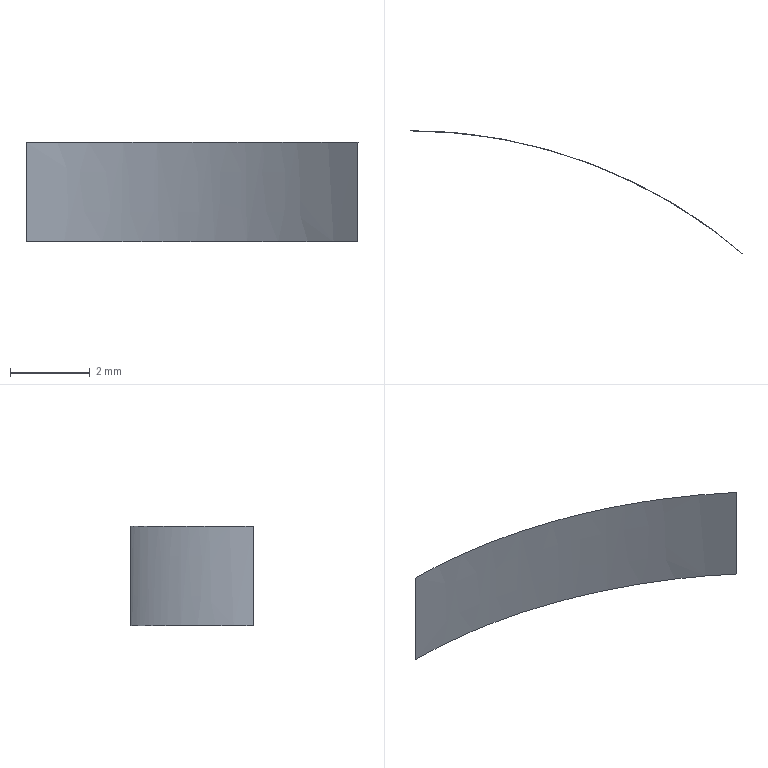Part | STEP file | lll_id370_x_t | 1 solid | 2 faces | box 8.307 x 3.062 x 2.5 mm | volume 0.01685 mm3 | other 1 | cylinder 1 | commonest cylinder face diameters 25.6 x1